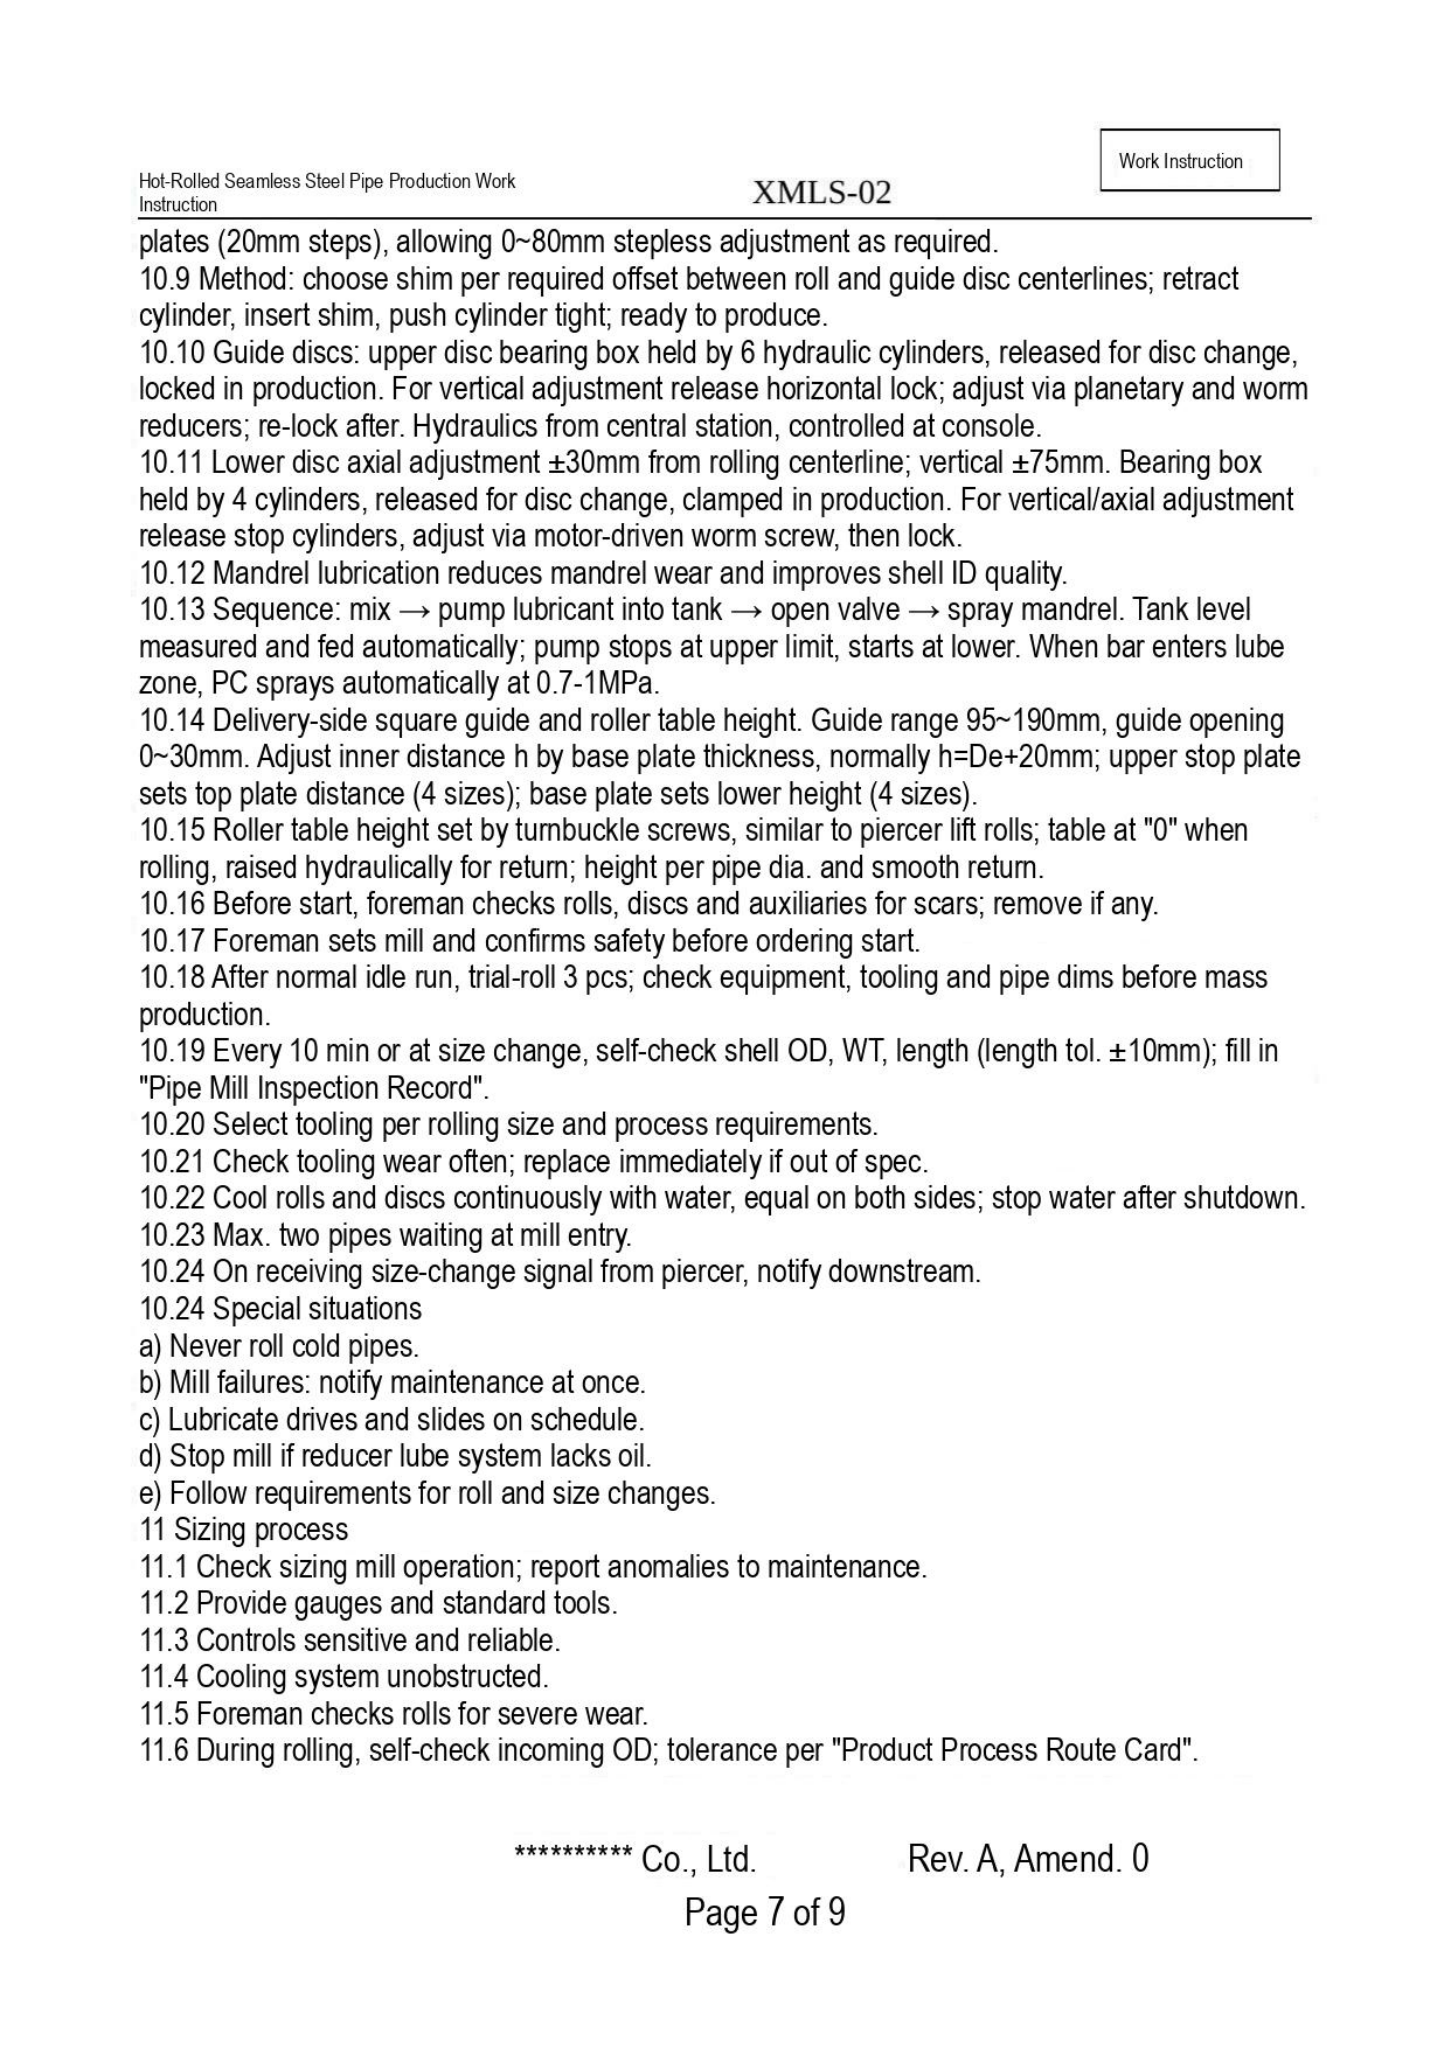Hot-Rolled Seamless Steel Pipe Production Work Instruction

XMLS-02

Work Instruction

plates (20mm steps), allowing 0~80mm stepless adjustment as required.
10.9 Method: choose shim per required offset between roll and guide disc centerlines; retract cylinder, insert shim, push cylinder tight; ready to produce.
10.10 Guide discs: upper disc bearing box held by 6 hydraulic cylinders, released for disc change, locked in production. For vertical adjustment release horizontal lock; adjust via planetary and worm reducers; re-lock after. Hydraulics from central station, controlled at console.
10.11 Lower disc axial adjustment ±30mm from rolling centerline; vertical ±75mm. Bearing box held by 4 cylinders, released for disc change, clamped in production. For vertical/axial adjustment release stop cylinders, adjust via motor-driven worm screw, then lock.
10.12 Mandrel lubrication reduces mandrel wear and improves shell ID quality.
10.13 Sequence: mix → pump lubricant into tank → open valve → spray mandrel. Tank level measured and fed automatically; pump stops at upper limit, starts at lower. When bar enters lube zone, PC sprays automatically at 0.7-1MPa.
10.14 Delivery-side square guide and roller table height. Guide range 95~190mm, guide opening 0~30mm. Adjust inner distance h by base plate thickness, normally h=De+20mm; upper stop plate sets top plate distance (4 sizes); base plate sets lower height (4 sizes).
10.15 Roller table height set by turnbuckle screws, similar to piercer lift rolls; table at "0" when rolling, raised hydraulically for return; height per pipe dia. and smooth return.
10.16 Before start, foreman checks rolls, discs and auxiliaries for scars; remove if any.
10.17 Foreman sets mill and confirms safety before ordering start.
10.18 After normal idle run, trial-roll 3 pcs; check equipment, tooling and pipe dims before mass production.
10.19 Every 10 min or at size change, self-check shell OD, WT, length (length tol. ±10mm); fill in "Pipe Mill Inspection Record".
10.20 Select tooling per rolling size and process requirements.
10.21 Check tooling wear often; replace immediately if out of spec.
10.22 Cool rolls and discs continuously with water, equal on both sides; stop water after shutdown.
10.23 Max. two pipes waiting at mill entry.
10.24 On receiving size-change signal from piercer, notify downstream.
10.24 Special situations
a) Never roll cold pipes.
b) Mill failures: notify maintenance at once.
c) Lubricate drives and slides on schedule.
d) Stop mill if reducer lube system lacks oil.
e) Follow requirements for roll and size changes.
11 Sizing process
11.1 Check sizing mill operation; report anomalies to maintenance.
11.2 Provide gauges and standard tools.
11.3 Controls sensitive and reliable.
11.4 Cooling system unobstructed.
11.5 Foreman checks rolls for severe wear.
11.6 During rolling, self-check incoming OD; tolerance per "Product Process Route Card".

********** Co., Ltd.    Rev. A, Amend. 0

Page 7 of 9
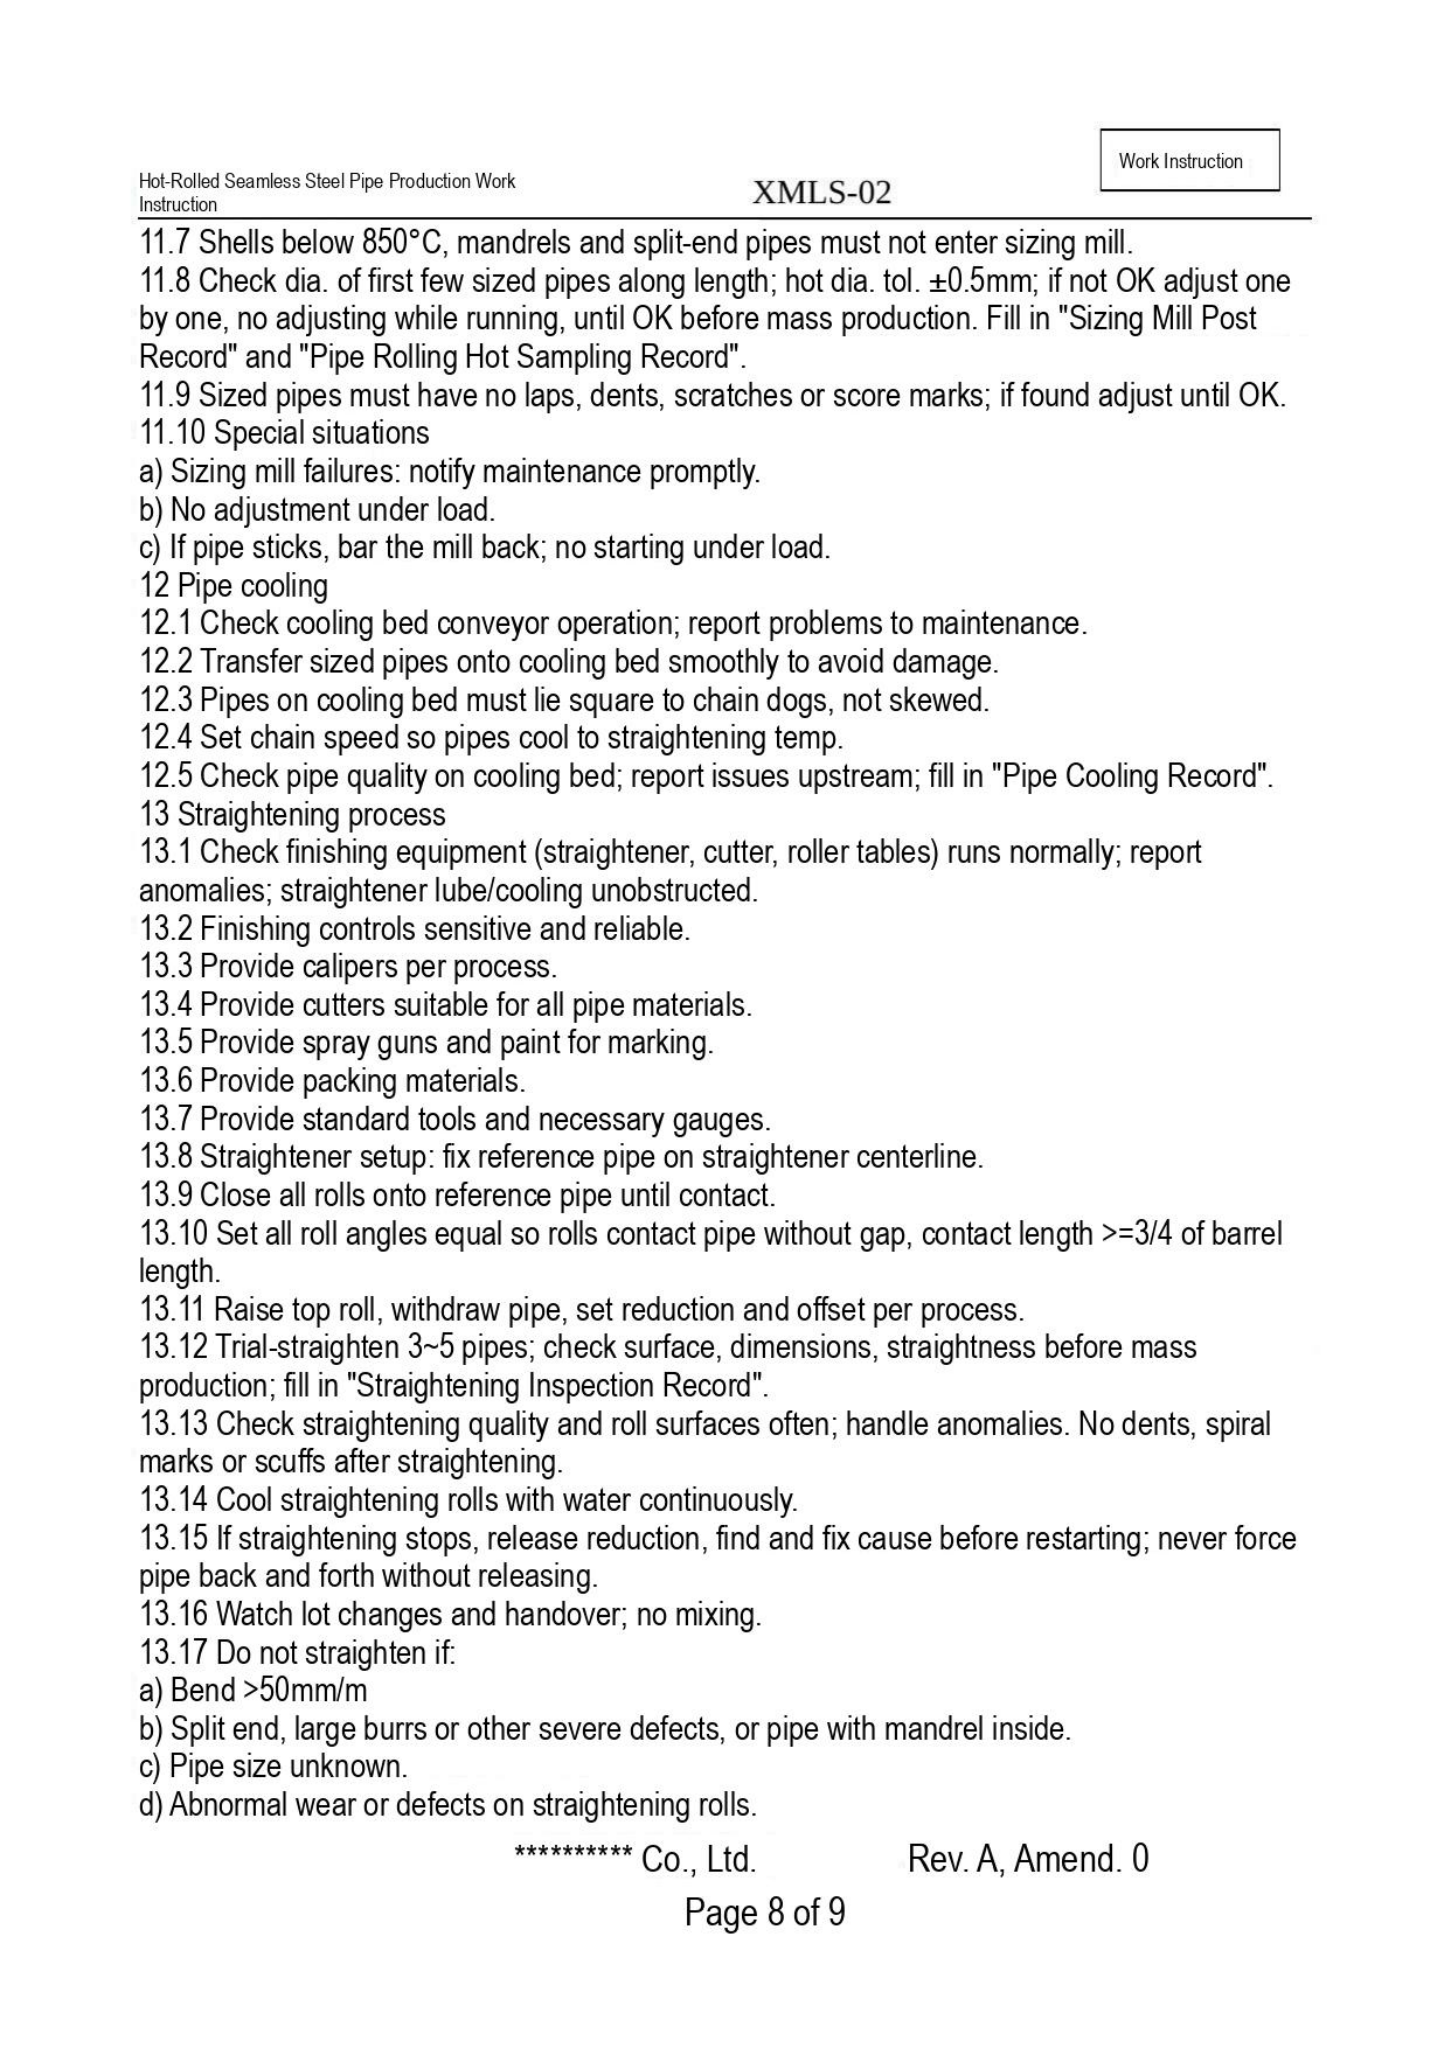Hot-Rolled Seamless Steel Pipe Production Work Instruction XMLS-02 Work Instruction

11.7 Shells below 850°C, mandrels and split-end pipes must not enter sizing mill.
11.8 Check dia. of first few sized pipes along length; hot dia. tol. ±0.5mm; if not OK adjust one by one, no adjusting while running, until OK before mass production. Fill in "Sizing Mill Post Record" and "Pipe Rolling Hot Sampling Record".
11.9 Sized pipes must have no laps, dents, scratches or score marks; if found adjust until OK.
11.10 Special situations
a) Sizing mill failures: notify maintenance promptly.
b) No adjustment under load.
c) If pipe sticks, bar the mill back; no starting under load.
12 Pipe cooling
12.1 Check cooling bed conveyor operation; report problems to maintenance.
12.2 Transfer sized pipes onto cooling bed smoothly to avoid damage.
12.3 Pipes on cooling bed must lie square to chain dogs, not skewed.
12.4 Set chain speed so pipes cool to straightening temp.
12.5 Check pipe quality on cooling bed; report issues upstream; fill in "Pipe Cooling Record".
13 Straightening process
13.1 Check finishing equipment (straightener, cutter, roller tables) runs normally; report anomalies; straightener lube/cooling unobstructed.
13.2 Finishing controls sensitive and reliable.
13.3 Provide calipers per process.
13.4 Provide cutters suitable for all pipe materials.
13.5 Provide spray guns and paint for marking.
13.6 Provide packing materials.
13.7 Provide standard tools and necessary gauges.
13.8 Straightener setup: fix reference pipe on straightener centerline.
13.9 Close all rolls onto reference pipe until contact.
13.10 Set all roll angles equal so rolls contact pipe without gap, contact length >=3/4 of barrel length.
13.11 Raise top roll, withdraw pipe, set reduction and offset per process.
13.12 Trial-straighten 3~5 pipes; check surface, dimensions, straightness before mass production; fill in "Straightening Inspection Record".
13.13 Check straightening quality and roll surfaces often; handle anomalies. No dents, spiral marks or scuffs after straightening.
13.14 Cool straightening rolls with water continuously.
13.15 If straightening stops, release reduction, find and fix cause before restarting; never force pipe back and forth without releasing.
13.16 Watch lot changes and handover; no mixing.
13.17 Do not straighten if:
a) Bend >50mm/m
b) Split end, large burrs or other severe defects, or pipe with mandrel inside.
c) Pipe size unknown.
d) Abnormal wear or defects on straightening rolls.

********** Co., Ltd. Rev. A, Amend. 0
Page 8 of 9
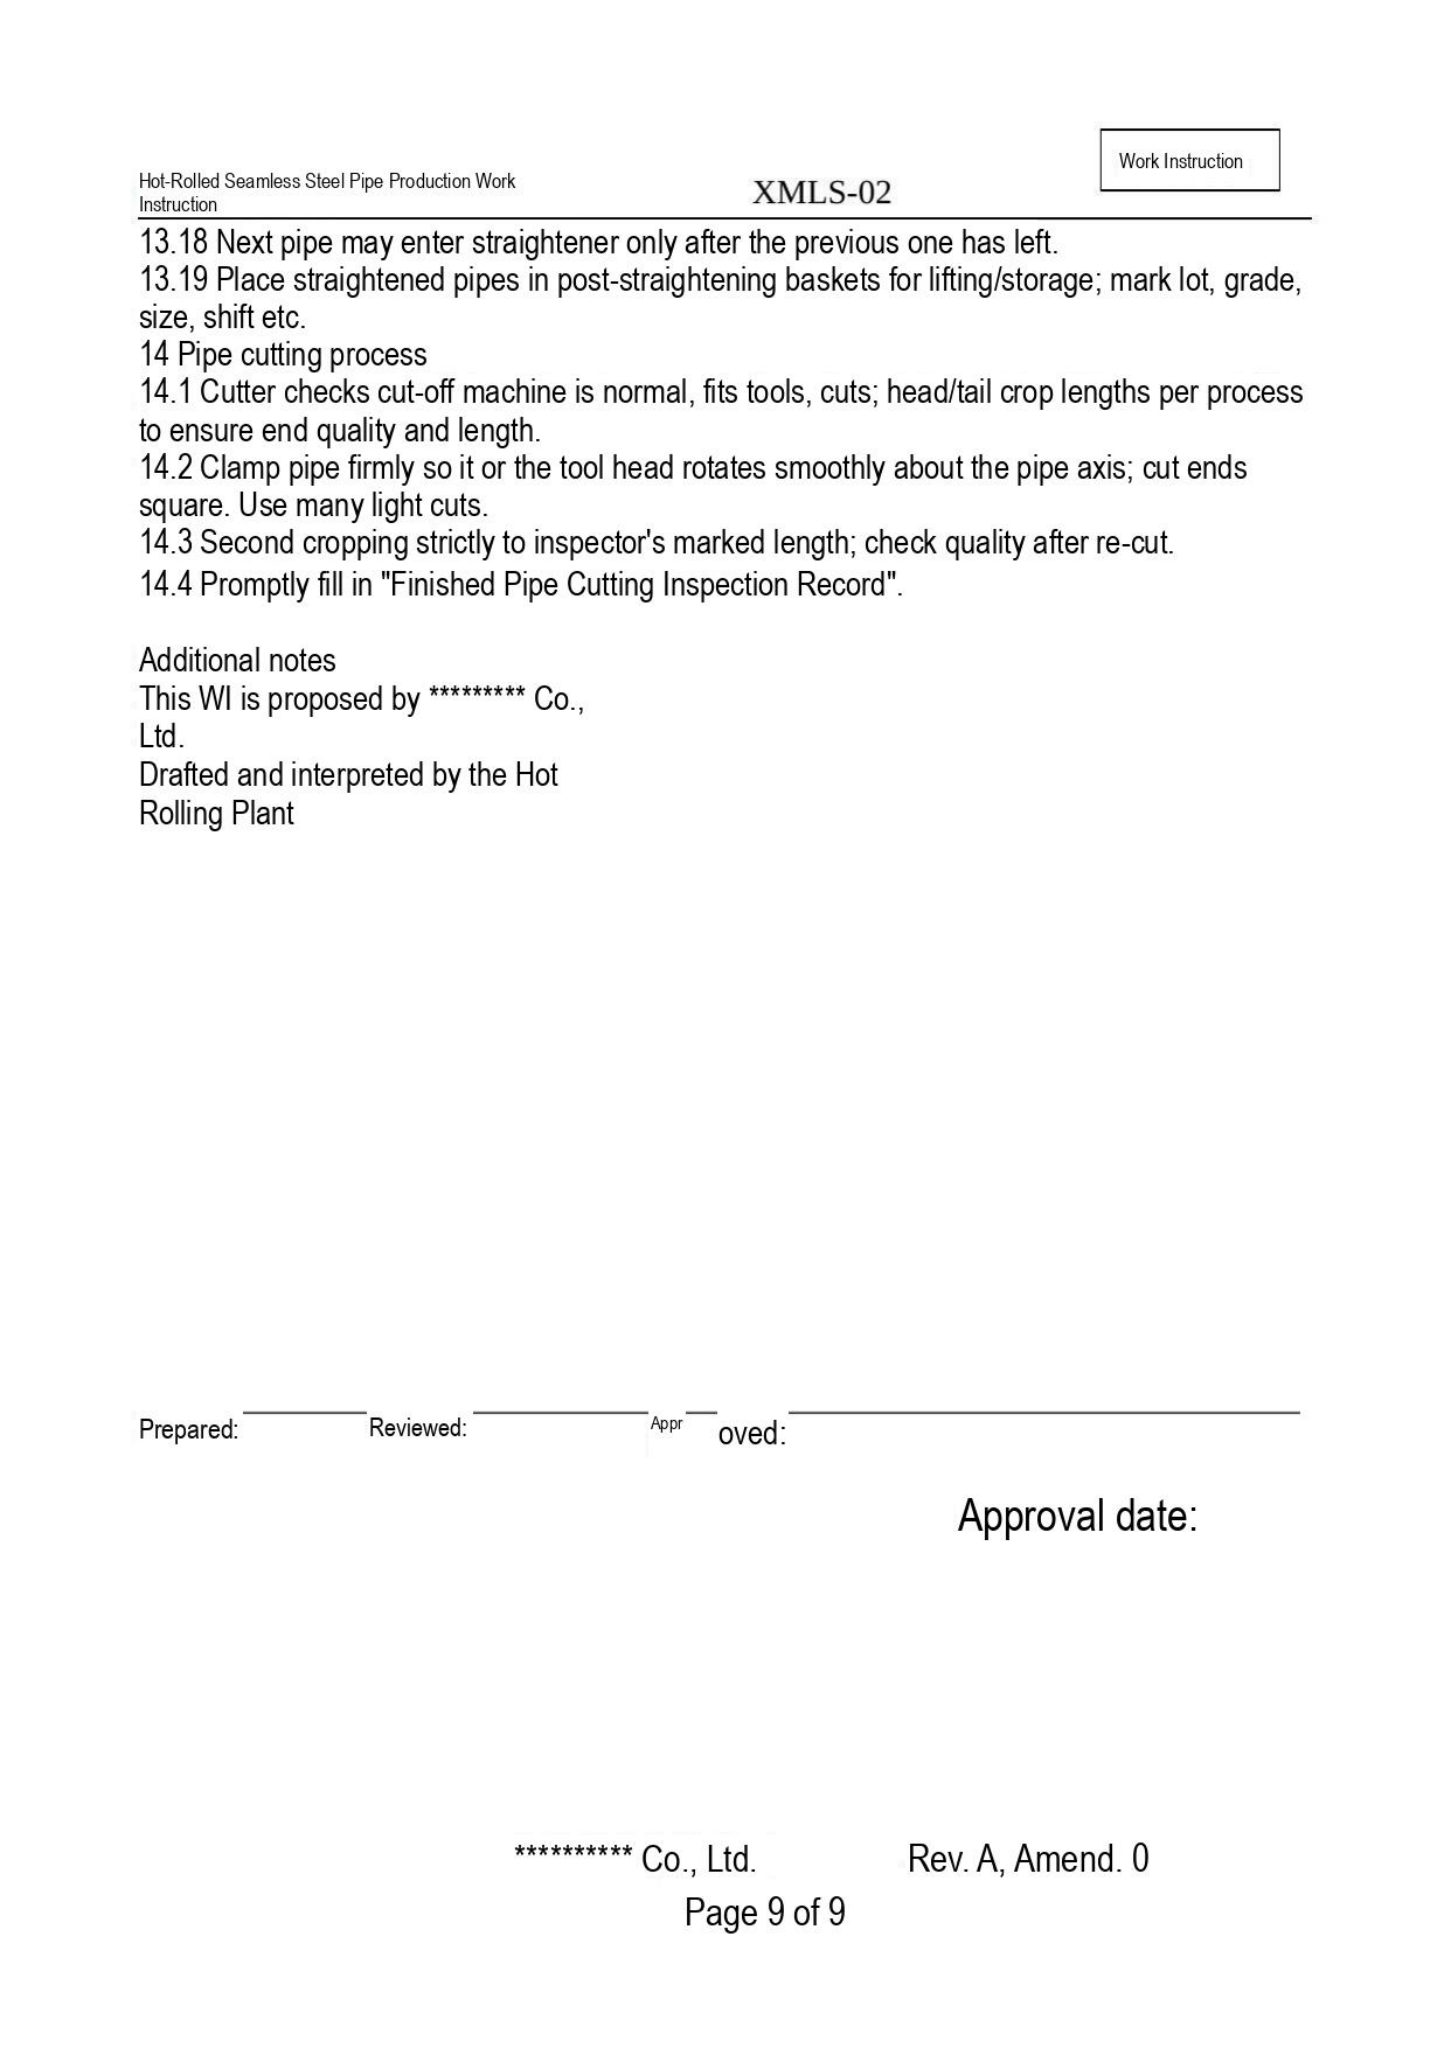Hot-Rolled Seamless Steel Pipe Production Work Instruction

XMLS-02

Work Instruction

13.18 Next pipe may enter straightener only after the previous one has left.
13.19 Place straightened pipes in post-straightening baskets for lifting/storage; mark lot, grade, size, shift etc.
14 Pipe cutting process
14.1 Cutter checks cut-off machine is normal, fits tools, cuts; head/tail crop lengths per process to ensure end quality and length.
14.2 Clamp pipe firmly so it or the tool head rotates smoothly about the pipe axis; cut ends square. Use many light cuts.
14.3 Second cropping strictly to inspector's marked length; check quality after re-cut.
14.4 Promptly fill in "Finished Pipe Cutting Inspection Record".

Additional notes
This WI is proposed by ********* Co., Ltd.
Drafted and interpreted by the Hot Rolling Plant

Prepared: Reviewed: Appr oved:

Approval date:

********** Co., Ltd. Rev. A, Amend. 0
Page 9 of 9